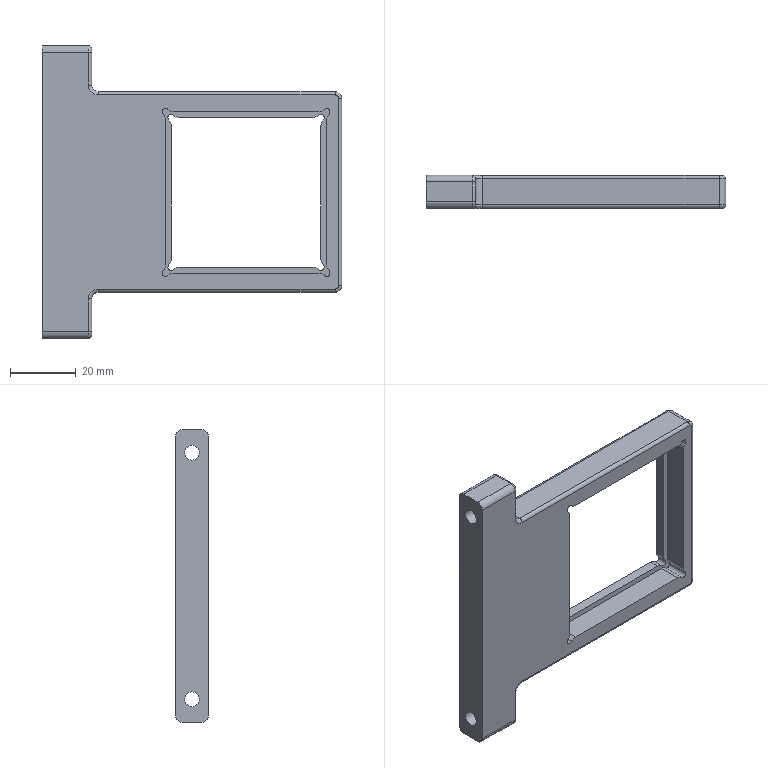NC program | NX | posted by the shop | part box 91 x 10 x 89 mm
Lines 2771 to 3778 of 16928:
N3 T04 M06
(D4  D=4. R=0. H=04 ce=0.05 di=0.05)
G00 G90 G54 X35.332 Y-21.985 M03 S6000
G43 H04 Z20.
M08
Z.31
G01 X35.333 Y-21.992 Z.225 F2000.
X35.336 Y-22.011 Z.147
X35.342 Y-22.04 Z.077
X35.35 Y-22.079 Z.014
X35.36 Y-22.124 Z-.041
X35.374 Y-22.175 Z-.09
X35.391 Y-22.229 Z-.133
X35.412 Y-22.285 Z-.17
X35.436 Y-22.341 Z-.201
X35.465 Y-22.395 Z-.226
X35.497 Y-22.446 Z-.247
X35.535 Y-22.491 Z-.263
X35.576 Y-22.529 Z-.275
X35.623 Y-22.559 Z-.283
X35.675 Y-22.578 Z-.288
X35.732 Y-22.585 Z-.29
X38.486 F2500.
G02 X38.904 Y-22.604 I0.0 J-4.55
X38.885 Y-22.185 I4.531 J.419
G01 Y-19.432
X38.869 Y-19.389
X38.823 Y-19.367 Z-.293
X38.751 Y-19.366 Z-.297
X38.656 Y-19.382 Z-.302
X38.541 Y-19.416 Z-.309
X38.411 Y-19.465 Z-.317
X38.267 Y-19.528 Z-.326
X38.115 Y-19.602 Z-.335
X37.956 Y-19.687 Z-.346
X37.795 Y-19.781 Z-.357
X37.635 Y-19.882 Z-.368
X37.298 Y-20.123 Z-.394
X36.982 Y-20.39 Z-.421
X36.691 Y-20.682 Z-.448
X36.423 Y-20.997 Z-.475
X36.182 Y-21.335 Z-.501
X36.081 Y-21.495 Z-.512
X35.987 Y-21.656 Z-.523
X35.903 Y-21.814 Z-.533
X35.828 Y-21.967 Z-.543
X35.765 Y-22.11 Z-.552
X35.717 Y-22.241 Z-.56
X35.683 Y-22.356 Z-.566
X35.666 Y-22.451 Z-.572
X35.667 Y-22.523 Z-.576
X35.689 Y-22.569 Z-.578
X35.732 Y-22.585 Z-.579
X38.486
G02 X38.904 Y-22.604 I0.0 J-4.55
X38.885 Y-22.185 I4.531 J.419
G01 Y-19.432
X38.869 Y-19.389 Z-.58
X38.823 Y-19.367 Z-.583
X38.751 Y-19.366 Z-.587
X38.656 Y-19.382 Z-.592
X38.541 Y-19.416 Z-.599
X38.411 Y-19.465 Z-.607
X38.267 Y-19.528 Z-.615
X38.115 Y-19.602 Z-.625
X37.956 Y-19.687 Z-.635
X37.795 Y-19.781 Z-.646
X37.635 Y-19.882 Z-.658
X37.298 Y-20.123 Z-.684
X36.982 Y-20.39 Z-.71
X36.691 Y-20.682 Z-.738
X36.423 Y-20.997 Z-.764
X36.182 Y-21.335 Z-.79
X36.081 Y-21.495 Z-.802
X35.987 Y-21.656 Z-.813
X35.903 Y-21.814 Z-.823
X35.828 Y-21.967 Z-.833
X35.765 Y-22.11 Z-.841
X35.717 Y-22.241 Z-.849
X35.683 Y-22.356 Z-.856
X35.666 Y-22.451 Z-.861
X35.667 Y-22.523 Z-.865
X35.689 Y-22.569 Z-.868
X35.732 Y-22.585 Z-.869
X38.486
G02 X38.904 Y-22.604 I0.0 J-4.55
X38.885 Y-22.185 I4.531 J.419
G01 Y-19.432
X38.869 Y-19.389 Z-.87
X38.823 Y-19.367 Z-.872
X38.751 Y-19.366 Z-.876
X38.656 Y-19.382 Z-.882
X38.541 Y-19.416 Z-.888
X38.411 Y-19.465 Z-.896
X38.267 Y-19.528 Z-.905
X38.115 Y-19.602 Z-.915
X37.956 Y-19.687 Z-.925
X37.795 Y-19.781 Z-.936
X37.635 Y-19.882 Z-.947
X37.298 Y-20.123 Z-.973
X36.982 Y-20.39 Z-1.
X36.691 Y-20.682 Z-1.027
X36.423 Y-20.997 Z-1.054
X36.182 Y-21.335 Z-1.08
X36.081 Y-21.495 Z-1.091
X35.987 Y-21.656 Z-1.102
X35.903 Y-21.814 Z-1.112
X35.828 Y-21.967 Z-1.122
X35.765 Y-22.11 Z-1.131
X35.717 Y-22.241 Z-1.139
X35.683 Y-22.356 Z-1.145
X35.666 Y-22.451 Z-1.151
X35.667 Y-22.523 Z-1.155
X35.689 Y-22.569 Z-1.157
X35.732 Y-22.585 Z-1.158
X38.486
G02 X38.904 Y-22.604 I0.0 J-4.55
X38.885 Y-22.185 I4.531 J.419
G01 Y-19.432
X38.869 Y-19.389 Z-1.159
X38.823 Y-19.367 Z-1.162
X38.751 Y-19.366 Z-1.166
X38.656 Y-19.382 Z-1.171
X38.541 Y-19.416 Z-1.178
X38.411 Y-19.465 Z-1.186
X38.267 Y-19.528 Z-1.195
X38.115 Y-19.602 Z-1.204
X37.956 Y-19.687 Z-1.215
X37.795 Y-19.781 Z-1.225
X37.635 Y-19.882 Z-1.237
X37.298 Y-20.123 Z-1.263
X36.982 Y-20.39 Z-1.29
X36.691 Y-20.682 Z-1.317
X36.423 Y-20.997 Z-1.344
X36.182 Y-21.335 Z-1.369
X36.081 Y-21.495 Z-1.381
X35.987 Y-21.656 Z-1.392
X35.903 Y-21.814 Z-1.402
X35.828 Y-21.967 Z-1.412
X35.765 Y-22.11 Z-1.421
X35.717 Y-22.241 Z-1.428
X35.683 Y-22.356 Z-1.435
X35.666 Y-22.451 Z-1.44
X35.667 Y-22.523 Z-1.445
X35.689 Y-22.569 Z-1.447
X35.732 Y-22.585 Z-1.448
X38.486
G02 X38.904 Y-22.604 I0.0 J-4.55
X38.885 Y-22.185 I4.531 J.419
G01 Y-19.432
X38.869 Y-19.389 Z-1.449
X38.823 Y-19.367 Z-1.451
X38.751 Y-19.366 Z-1.455
X38.656 Y-19.382 Z-1.461
X38.541 Y-19.416 Z-1.468
X38.411 Y-19.465 Z-1.475
X38.267 Y-19.528 Z-1.484
X38.115 Y-19.602 Z-1.494
X37.956 Y-19.687 Z-1.504
X37.795 Y-19.781 Z-1.515
X37.635 Y-19.882 Z-1.526
X37.298 Y-20.123 Z-1.552
X36.982 Y-20.39 Z-1.579
X36.691 Y-20.682 Z-1.606
X36.423 Y-20.997 Z-1.633
X36.182 Y-21.335 Z-1.659
X36.081 Y-21.495 Z-1.67
X35.987 Y-21.656 Z-1.681
X35.903 Y-21.814 Z-1.692
X35.828 Y-21.967 Z-1.701
X35.765 Y-22.11 Z-1.71
X35.717 Y-22.241 Z-1.718
X35.683 Y-22.356 Z-1.725
X35.666 Y-22.451 Z-1.73
X35.667 Y-22.523 Z-1.734
X35.689 Y-22.569 Z-1.737
X35.732 Y-22.585 Z-1.738
X38.486
G02 X38.904 Y-22.604 I0.0 J-4.55
X38.885 Y-22.185 I4.531 J.419
G01 Y-19.432
X38.869 Y-19.389
X38.823 Y-19.367 Z-1.741
X38.751 Y-19.366 Z-1.745
X38.656 Y-19.382 Z-1.75
X38.541 Y-19.416 Z-1.757
X38.411 Y-19.465 Z-1.765
X38.267 Y-19.528 Z-1.774
X38.115 Y-19.602 Z-1.783
X37.956 Y-19.687 Z-1.794
X37.795 Y-19.781 Z-1.805
X37.635 Y-19.882 Z-1.816
X37.298 Y-20.123 Z-1.842
X36.982 Y-20.39 Z-1.869
X36.691 Y-20.682 Z-1.896
X36.423 Y-20.997 Z-1.923
X36.182 Y-21.335 Z-1.949
X36.081 Y-21.495 Z-1.96
X35.987 Y-21.656 Z-1.971
X35.903 Y-21.814 Z-1.981
X35.828 Y-21.967 Z-1.991
X35.765 Y-22.11 Z-2.
X35.717 Y-22.241 Z-2.007
X35.683 Y-22.356 Z-2.014
X35.666 Y-22.451 Z-2.02
X35.667 Y-22.523 Z-2.024
X35.689 Y-22.569 Z-2.026
X35.732 Y-22.585 Z-2.027
X38.486
G02 X38.904 Y-22.604 I0.0 J-4.55
X38.885 Y-22.185 I4.531 J.419
G01 Y-19.432
X38.869 Y-19.389 Z-2.028
X38.823 Y-19.367 Z-2.03
X38.751 Y-19.366 Z-2.035
X38.656 Y-19.382 Z-2.04
X38.541 Y-19.416 Z-2.047
X38.411 Y-19.465 Z-2.054
X38.267 Y-19.528 Z-2.063
X38.115 Y-19.602 Z-2.073
X37.956 Y-19.687 Z-2.083
X37.795 Y-19.781 Z-2.094
X37.635 Y-19.882 Z-2.106
X37.298 Y-20.123 Z-2.131
X36.982 Y-20.39 Z-2.158
X36.691 Y-20.682 Z-2.185
X36.423 Y-20.997 Z-2.212
X36.182 Y-21.335 Z-2.238
X36.081 Y-21.495 Z-2.25
X35.987 Y-21.656 Z-2.26
X35.903 Y-21.814 Z-2.271
X35.828 Y-21.967 Z-2.28
X35.765 Y-22.11 Z-2.289
X35.717 Y-22.241 Z-2.297
X35.683 Y-22.356 Z-2.304
X35.666 Y-22.451 Z-2.309
X35.667 Y-22.523 Z-2.313
X35.689 Y-22.569 Z-2.316
X35.732 Y-22.585 Z-2.317
X38.486
G02 X38.904 Y-22.604 I0.0 J-4.55
X38.885 Y-22.185 I4.531 J.419
G01 Y-19.432
X38.869 Y-19.389 Z-2.318
X38.823 Y-19.367 Z-2.32
X38.751 Y-19.366 Z-2.324
X38.656 Y-19.382 Z-2.33
X38.541 Y-19.416 Z-2.336
X38.411 Y-19.465 Z-2.344
X38.267 Y-19.528 Z-2.353
X38.115 Y-19.602 Z-2.363
X37.956 Y-19.687 Z-2.373
X37.795 Y-19.781 Z-2.384
X37.635 Y-19.882 Z-2.395
X37.298 Y-20.123 Z-2.421
X36.982 Y-20.39 Z-2.448
X36.691 Y-20.682 Z-2.475
X36.423 Y-20.997 Z-2.502
X36.182 Y-21.335 Z-2.528
X36.081 Y-21.495 Z-2.539
X35.987 Y-21.656 Z-2.55
X35.903 Y-21.814 Z-2.56
X35.828 Y-21.967 Z-2.57
X35.765 Y-22.11 Z-2.579
X35.717 Y-22.241 Z-2.587
X35.683 Y-22.356 Z-2.593
X35.666 Y-22.451 Z-2.599
X35.667 Y-22.523 Z-2.603
X35.689 Y-22.569 Z-2.605
X35.732 Y-22.585 Z-2.606
X38.486
G02 X38.904 Y-22.604 I0.0 J-4.55
X38.885 Y-22.185 I4.531 J.419
G01 Y-19.432
X38.869 Y-19.389 Z-2.607
X38.823 Y-19.367 Z-2.61
X38.751 Y-19.366 Z-2.614
X38.656 Y-19.382 Z-2.619
X38.541 Y-19.416 Z-2.626
X38.411 Y-19.465 Z-2.634
X38.267 Y-19.528 Z-2.642
X38.115 Y-19.602 Z-2.652
X37.956 Y-19.687 Z-2.662
X37.795 Y-19.781 Z-2.673
X37.635 Y-19.882 Z-2.685
X37.298 Y-20.123 Z-2.711
X36.982 Y-20.39 Z-2.737
X36.691 Y-20.682 Z-2.765
X36.423 Y-20.997 Z-2.791
X36.182 Y-21.335 Z-2.817
X36.081 Y-21.495 Z-2.829
X35.987 Y-21.656 Z-2.84
X35.903 Y-21.814 Z-2.85
X35.828 Y-21.967 Z-2.86
X35.765 Y-22.11 Z-2.868
X35.717 Y-22.241 Z-2.876
X35.683 Y-22.356 Z-2.883
X35.666 Y-22.451 Z-2.888
X35.667 Y-22.523 Z-2.892
X35.689 Y-22.569 Z-2.895
X35.732 Y-22.585 Z-2.896
X38.486
G02 X38.904 Y-22.604 I0.0 J-4.55
X38.885 Y-22.185 I4.531 J.419
G01 Y-19.432
X38.869 Y-19.389 Z-2.897
X38.823 Y-19.367 Z-2.899
X38.751 Y-19.366 Z-2.903
X38.656 Y-19.382 Z-2.909
X38.541 Y-19.416 Z-2.915
X38.411 Y-19.465 Z-2.923
X38.267 Y-19.528 Z-2.932
X38.115 Y-19.602 Z-2.942
X37.956 Y-19.687 Z-2.952
X37.795 Y-19.781 Z-2.963
X37.635 Y-19.882 Z-2.974
X37.298 Y-20.123 Z-3.
X36.982 Y-20.39 Z-3.027
X36.691 Y-20.682 Z-3.054
X36.423 Y-20.997 Z-3.081
X36.182 Y-21.335 Z-3.107
X36.081 Y-21.495 Z-3.118
X35.987 Y-21.656 Z-3.129
X35.903 Y-21.814 Z-3.14
X35.828 Y-21.967 Z-3.149
X35.765 Y-22.11 Z-3.158
X35.717 Y-22.241 Z-3.166
X35.683 Y-22.356 Z-3.173
X35.666 Y-22.451 Z-3.178
X35.667 Y-22.523 Z-3.182
X35.689 Y-22.569 Z-3.185
X35.732 Y-22.585
X38.486
G02 X38.904 Y-22.604 I0.0 J-4.55
X38.885 Y-22.185 I4.531 J.419
G01 Y-19.432
X38.869 Y-19.389 Z-3.186
X38.823 Y-19.367 Z-3.189
X38.751 Y-19.366 Z-3.193
X38.656 Y-19.382 Z-3.198
X38.541 Y-19.416 Z-3.205
X38.411 Y-19.465 Z-3.213
X38.267 Y-19.528 Z-3.222
X38.115 Y-19.602 Z-3.231
X37.956 Y-19.687 Z-3.242
X37.795 Y-19.781 Z-3.253
X37.635 Y-19.882 Z-3.264
X37.298 Y-20.123 Z-3.29
X36.982 Y-20.39 Z-3.317
X36.691 Y-20.682 Z-3.344
X36.423 Y-20.997 Z-3.371
X36.182 Y-21.335 Z-3.397
X36.081 Y-21.495 Z-3.408
X35.987 Y-21.656 Z-3.419
X35.903 Y-21.814 Z-3.429
X35.828 Y-21.967 Z-3.439
X35.765 Y-22.11 Z-3.448
X35.717 Y-22.241 Z-3.455
X35.683 Y-22.356 Z-3.462
X35.666 Y-22.451 Z-3.468
X35.667 Y-22.523 Z-3.472
X35.689 Y-22.569 Z-3.474
X35.732 Y-22.585 Z-3.475
X38.486
G02 X38.904 Y-22.604 I0.0 J-4.55
X38.885 Y-22.185 I4.531 J.419
G01 Y-19.432
X38.869 Y-19.389 Z-3.476
X38.823 Y-19.367 Z-3.478
X38.751 Y-19.366 Z-3.482
X38.656 Y-19.382 Z-3.488
X38.541 Y-19.416 Z-3.495
X38.411 Y-19.465 Z-3.502
X38.267 Y-19.528 Z-3.511
X38.115 Y-19.602 Z-3.521
X37.956 Y-19.687 Z-3.531
X37.795 Y-19.781 Z-3.542
X37.635 Y-19.882 Z-3.553
X37.298 Y-20.123 Z-3.579
X36.982 Y-20.39 Z-3.606
X36.691 Y-20.682 Z-3.633
X36.423 Y-20.997 Z-3.66
X36.182 Y-21.335 Z-3.686
X36.081 Y-21.495 Z-3.698
X35.987 Y-21.656 Z-3.708
X35.903 Y-21.814 Z-3.719
X35.828 Y-21.967 Z-3.728
X35.765 Y-22.11 Z-3.737
X35.717 Y-22.241 Z-3.745
X35.683 Y-22.356 Z-3.752
X35.666 Y-22.451 Z-3.757
X35.667 Y-22.523 Z-3.761
X35.689 Y-22.569 Z-3.764
X35.732 Y-22.585 Z-3.765
X38.486
G02 X38.904 Y-22.604 I0.0 J-4.55
X38.885 Y-22.185 I4.531 J.419
G01 Y-19.432
X38.869 Y-19.389
X38.823 Y-19.367 Z-3.768
X38.751 Y-19.366 Z-3.772
X38.656 Y-19.382 Z-3.777
X38.541 Y-19.416 Z-3.784
X38.411 Y-19.465 Z-3.792
X38.267 Y-19.528 Z-3.801
X38.115 Y-19.602 Z-3.81
X37.956 Y-19.687 Z-3.821
X37.795 Y-19.781 Z-3.832
X37.635 Y-19.882 Z-3.843
X37.298 Y-20.123 Z-3.869
X36.982 Y-20.39 Z-3.896
X36.691 Y-20.682 Z-3.923
X36.423 Y-20.997 Z-3.95
X36.182 Y-21.335 Z-3.976
X36.081 Y-21.495 Z-3.987
X35.987 Y-21.656 Z-3.998
X35.903 Y-21.814 Z-4.008
X35.828 Y-21.967 Z-4.018
X35.765 Y-22.11 Z-4.027
X35.717 Y-22.241 Z-4.035
X35.683 Y-22.356 Z-4.041
X35.666 Y-22.451 Z-4.047
X35.667 Y-22.523 Z-4.051
X35.689 Y-22.569 Z-4.053
X35.732 Y-22.585 Z-4.054
X38.486
G02 X38.904 Y-22.604 I0.0 J-4.55
X38.885 Y-22.185 I4.531 J.419
G01 Y-19.432
X38.869 Y-19.389 Z-4.055
X38.823 Y-19.367 Z-4.058
X38.751 Y-19.366 Z-4.062
X38.656 Y-19.382 Z-4.067
X38.541 Y-19.416 Z-4.074
X38.411 Y-19.465 Z-4.082
X38.267 Y-19.528 Z-4.09
X38.115 Y-19.602 Z-4.1
X37.956 Y-19.687 Z-4.11
X37.795 Y-19.781 Z-4.121
X37.635 Y-19.882 Z-4.133
X37.298 Y-20.123 Z-4.159
X36.982 Y-20.39 Z-4.185
X36.691 Y-20.682 Z-4.213
X36.423 Y-20.997 Z-4.239
X36.182 Y-21.335 Z-4.265
X36.081 Y-21.495 Z-4.277
X35.987 Y-21.656 Z-4.288
X35.903 Y-21.814 Z-4.298
X35.828 Y-21.967 Z-4.308
X35.765 Y-22.11 Z-4.316
X35.717 Y-22.241 Z-4.324
X35.683 Y-22.356 Z-4.331
X35.666 Y-22.451 Z-4.336
X35.667 Y-22.523 Z-4.34
X35.689 Y-22.569 Z-4.343
X35.732 Y-22.585 Z-4.344
X38.486
G02 X38.904 Y-22.604 I0.0 J-4.55
X38.885 Y-22.185 I4.531 J.419
G01 Y-19.432
X38.869 Y-19.389 Z-4.345
X38.823 Y-19.367 Z-4.347
X38.751 Y-19.366 Z-4.351
X38.656 Y-19.382 Z-4.357
X38.541 Y-19.416 Z-4.363
X38.411 Y-19.465 Z-4.371
X38.267 Y-19.528 Z-4.38
X38.115 Y-19.602 Z-4.39
X37.956 Y-19.687 Z-4.4
X37.795 Y-19.781 Z-4.411
X37.635 Y-19.882 Z-4.422
X37.298 Y-20.123 Z-4.448
X36.982 Y-20.39 Z-4.475
X36.691 Y-20.682 Z-4.502
X36.423 Y-20.997 Z-4.529
X36.182 Y-21.335 Z-4.555
X36.081 Y-21.495 Z-4.566
X35.987 Y-21.656 Z-4.577
X35.903 Y-21.814 Z-4.587
X35.828 Y-21.967 Z-4.597
X35.765 Y-22.11 Z-4.606
X35.717 Y-22.241 Z-4.614
X35.683 Y-22.356 Z-4.62
X35.666 Y-22.451 Z-4.626
X35.667 Y-22.523 Z-4.63
X35.689 Y-22.569 Z-4.632
X35.732 Y-22.585 Z-4.633
X38.486
G02 X38.904 Y-22.604 I0.0 J-4.55
X38.885 Y-22.185 I4.531 J.419
G01 Y-19.432
X38.869 Y-19.389 Z-4.634
X38.823 Y-19.367 Z-4.637
X38.751 Y-19.366 Z-4.641
X38.656 Y-19.382 Z-4.646
X38.541 Y-19.416 Z-4.653
X38.411 Y-19.465 Z-4.661
X38.267 Y-19.528 Z-4.67
X38.115 Y-19.602 Z-4.679
X37.956 Y-19.687 Z-4.69
X37.795 Y-19.781 Z-4.7
X37.635 Y-19.882 Z-4.712
X37.298 Y-20.123 Z-4.738
X36.982 Y-20.39 Z-4.765
X36.691 Y-20.682 Z-4.792
X36.423 Y-20.997 Z-4.819
X36.182 Y-21.335 Z-4.844
X36.081 Y-21.495 Z-4.856
X35.987 Y-21.656 Z-4.867
X35.903 Y-21.814 Z-4.877
X35.828 Y-21.967 Z-4.887
X35.765 Y-22.11 Z-4.896
X35.717 Y-22.241 Z-4.903
X35.683 Y-22.356 Z-4.91
X35.666 Y-22.451 Z-4.915
X35.667 Y-22.523 Z-4.92
X35.689 Y-22.569 Z-4.922
X35.732 Y-22.585 Z-4.923
X38.486
G02 X38.904 Y-22.604 I0.0 J-4.55
X38.885 Y-22.185 I4.531 J.419
G01 Y-19.432
X38.869 Y-19.389 Z-4.924
X38.823 Y-19.367 Z-4.926
X38.751 Y-19.366 Z-4.93
X38.656 Y-19.382 Z-4.936
X38.541 Y-19.416 Z-4.943
X38.411 Y-19.465 Z-4.95
X38.267 Y-19.528 Z-4.959
X38.115 Y-19.602 Z-4.969
X37.956 Y-19.687 Z-4.979
X37.795 Y-19.781 Z-4.99
X37.635 Y-19.882 Z-5.001
X37.298 Y-20.123 Z-5.027
X36.982 Y-20.39 Z-5.054
X36.691 Y-20.682 Z-5.081
X36.423 Y-20.997 Z-5.108
X36.182 Y-21.335 Z-5.134
X36.081 Y-21.495 Z-5.145
X35.987 Y-21.656 Z-5.156
X35.903 Y-21.814 Z-5.167
X35.828 Y-21.967 Z-5.176
X35.765 Y-22.11 Z-5.185
X35.717 Y-22.241 Z-5.193
X35.683 Y-22.356 Z-5.2
X35.666 Y-22.451 Z-5.205
X35.667 Y-22.523 Z-5.209
X35.689 Y-22.569 Z-5.212
X35.732 Y-22.585 Z-5.213
X38.486
G02 X38.904 Y-22.604 I0.0 J-4.55
X38.885 Y-22.185 I4.531 J.419
G01 Y-19.432
X38.869 Y-19.389
X38.823 Y-19.367 Z-5.216
X38.751 Y-19.366 Z-5.22
X38.656 Y-19.382 Z-5.225
X38.541 Y-19.416 Z-5.232
X38.411 Y-19.465 Z-5.24
X38.267 Y-19.528 Z-5.249
X38.115 Y-19.602 Z-5.258
X37.956 Y-19.687 Z-5.269
X37.795 Y-19.781 Z-5.28
X37.635 Y-19.882 Z-5.291
X37.298 Y-20.123 Z-5.317
X36.982 Y-20.39 Z-5.344
X36.691 Y-20.682 Z-5.371
X36.423 Y-20.997 Z-5.398
X36.182 Y-21.335 Z-5.424
X36.081 Y-21.495 Z-5.435
X35.987 Y-21.656 Z-5.446
X35.903 Y-21.814 Z-5.456
X35.828 Y-21.967 Z-5.466
X35.765 Y-22.11 Z-5.475
X35.717 Y-22.241 Z-5.482
X35.683 Y-22.356 Z-5.489
X35.666 Y-22.451 Z-5.495
X35.667 Y-22.523 Z-5.499
X35.689 Y-22.569 Z-5.501
X35.732 Y-22.585 Z-5.502
X38.486
G02 X38.904 Y-22.604 I0.0 J-4.55
X38.885 Y-22.185 I4.531 J.419
G01 Y-19.432
X38.869 Y-19.389 Z-5.503
X38.823 Y-19.367 Z-5.505
X38.751 Y-19.366 Z-5.51
X38.656 Y-19.382 Z-5.515
X38.541 Y-19.416 Z-5.522
X38.411 Y-19.465 Z-5.529
X38.267 Y-19.528 Z-5.538
X38.115 Y-19.602 Z-5.548
X37.956 Y-19.687 Z-5.558
X37.795 Y-19.781 Z-5.569
X37.635 Y-19.882 Z-5.581
X37.298 Y-20.123 Z-5.606
X36.982 Y-20.39 Z-5.633
X36.691 Y-20.682 Z-5.66
X36.423 Y-20.997 Z-5.687
X36.182 Y-21.335 Z-5.713
X36.081 Y-21.495 Z-5.725
X35.987 Y-21.656 Z-5.735
X35.903 Y-21.814 Z-5.746
X35.828 Y-21.967 Z-5.755
X35.765 Y-22.11 Z-5.764
X35.717 Y-22.241 Z-5.772
X35.683 Y-22.356 Z-5.779
X35.666 Y-22.451 Z-5.784
X35.667 Y-22.523 Z-5.788
X35.689 Y-22.569 Z-5.791
X35.732 Y-22.585 Z-5.792
X38.486
G02 X38.904 Y-22.604 I0.0 J-4.55
X38.885 Y-22.185 I4.531 J.419
G01 Y-19.432
X38.869 Y-19.389 Z-5.793
X38.823 Y-19.367 Z-5.795
X38.751 Y-19.366 Z-5.799
X38.656 Y-19.382 Z-5.805
X38.541 Y-19.416 Z-5.811
X38.411 Y-19.465 Z-5.819
X38.267 Y-19.528 Z-5.828
X38.115 Y-19.602 Z-5.838
X37.956 Y-19.687 Z-5.848
X37.795 Y-19.781 Z-5.859
X37.635 Y-19.882 Z-5.87
X37.298 Y-20.123 Z-5.896
X36.982 Y-20.39 Z-5.923
X36.691 Y-20.682 Z-5.95
X36.423 Y-20.997 Z-5.977
X36.182 Y-21.335 Z-6.003
X36.081 Y-21.495 Z-6.014
X35.987 Y-21.656 Z-6.025
X35.903 Y-21.814 Z-6.035
X35.828 Y-21.967 Z-6.045
X35.765 Y-22.11 Z-6.054
X35.717 Y-22.241 Z-6.062
X35.683 Y-22.356 Z-6.068
X35.666 Y-22.451 Z-6.074
X35.667 Y-22.523 Z-6.078
X35.689 Y-22.569 Z-6.08
X35.732 Y-22.585 Z-6.081
X38.486
G02 X38.904 Y-22.604 I0.0 J-4.55
X38.885 Y-22.185 I4.531 J.419
G01 Y-19.432
X38.869 Y-19.389 Z-6.082
X38.823 Y-19.367 Z-6.085
X38.751 Y-19.366 Z-6.089
X38.656 Y-19.382 Z-6.094
X38.541 Y-19.416 Z-6.101
X38.411 Y-19.465 Z-6.109
X38.267 Y-19.528 Z-6.117
X38.115 Y-19.602 Z-6.127
X37.956 Y-19.687 Z-6.137
X37.795 Y-19.781 Z-6.148
X37.635 Y-19.882 Z-6.16
X37.298 Y-20.123 Z-6.186
X36.982 Y-20.39 Z-6.212
X36.691 Y-20.682 Z-6.24
X36.423 Y-20.997 Z-6.266
X36.182 Y-21.335 Z-6.292
X36.081 Y-21.495 Z-6.304
X35.987 Y-21.656 Z-6.315
X35.903 Y-21.814 Z-6.325
X35.828 Y-21.967 Z-6.335
X35.765 Y-22.11 Z-6.343
X35.717 Y-22.241 Z-6.351
X35.683 Y-22.356 Z-6.358
X35.666 Y-22.451 Z-6.363
X35.667 Y-22.523 Z-6.367
X35.689 Y-22.569 Z-6.37
X35.732 Y-22.585 Z-6.371
X38.486
G02 X38.904 Y-22.604 I0.0 J-4.55
X38.885 Y-22.185 I4.531 J.419
G01 Y-19.432
X38.869 Y-19.389 Z-6.372
X38.823 Y-19.367 Z-6.374
X38.751 Y-19.366 Z-6.378
X38.656 Y-19.382 Z-6.384
X38.541 Y-19.416 Z-6.39
X38.411 Y-19.465 Z-6.398
X38.267 Y-19.528 Z-6.407
X38.115 Y-19.602 Z-6.417
X37.956 Y-19.687 Z-6.427
X37.795 Y-19.781 Z-6.438
X37.635 Y-19.882 Z-6.449
X37.298 Y-20.123 Z-6.475
X36.982 Y-20.39 Z-6.502
X36.691 Y-20.682 Z-6.529
X36.423 Y-20.997 Z-6.556
X36.182 Y-21.335 Z-6.582
X36.081 Y-21.495 Z-6.593
X35.987 Y-21.656 Z-6.604
X35.903 Y-21.814 Z-6.615
X35.828 Y-21.967 Z-6.624
X35.765 Y-22.11 Z-6.633
X35.717 Y-22.241 Z-6.641
X35.683 Y-22.356 Z-6.648
X35.666 Y-22.451 Z-6.653
X35.667 Y-22.523 Z-6.657
X35.689 Y-22.569 Z-6.66
X35.732 Y-22.585
X38.486
G02 X38.904 Y-22.604 I0.0 J-4.55
X38.885 Y-22.185 I4.531 J.419
G01 Y-19.432
X38.869 Y-19.389 Z-6.661
X38.823 Y-19.367 Z-6.664
X38.751 Y-19.366 Z-6.668
X38.656 Y-19.382 Z-6.673
X38.541 Y-19.416 Z-6.68
X38.411 Y-19.465 Z-6.688
X38.267 Y-19.528 Z-6.697
X38.115 Y-19.602 Z-6.706
X37.956 Y-19.687 Z-6.717
X37.795 Y-19.781 Z-6.728
X37.635 Y-19.882 Z-6.739
X37.298 Y-20.123 Z-6.765
X36.982 Y-20.39 Z-6.792
X36.691 Y-20.682 Z-6.819
X36.423 Y-20.997 Z-6.846
X36.182 Y-21.335 Z-6.872
X36.081 Y-21.495 Z-6.883
X35.987 Y-21.656 Z-6.894
X35.903 Y-21.814 Z-6.904
X35.828 Y-21.967 Z-6.914
X35.765 Y-22.11 Z-6.923
X35.717 Y-22.241 Z-6.93
X35.683 Y-22.356 Z-6.937
X35.666 Y-22.451 Z-6.943
X35.667 Y-22.523 Z-6.947
X35.689 Y-22.569 Z-6.949
X35.732 Y-22.585 Z-6.95
X38.486
G02 X38.904 Y-22.604 I0.0 J-4.55
X38.885 Y-22.185 I4.531 J.419
G01 Y-19.432
X38.878 Y-19.375 Z-6.949
X38.859 Y-19.323 Z-6.944
X38.83 Y-19.276 Z-6.936
X38.791 Y-19.234 Z-6.924
X38.746 Y-19.197 Z-6.908
X38.695 Y-19.165 Z-6.887
X38.641 Y-19.136 Z-6.861
X38.585 Y-19.112 Z-6.83
X38.529 Y-19.091 Z-6.793
X38.475 Y-19.074 Z-6.751
X38.424 Y-19.06 Z-6.702
X38.379 Y-19.049 Z-6.646
X38.34 Y-19.041 Z-6.584
X38.311 Y-19.036 Z-6.514
X38.292 Y-19.033 Z-6.436
X38.285 Y-19.032 Z-6.35
G00 Z3.
Y18.762
Z.31
G01 X38.292 Y18.763 Z.225 F2000.
X38.311 Y18.766 Z.147
X38.34 Y18.772 Z.077
X38.379 Y18.78 Z.014
X38.424 Y18.791 Z-.041
X38.475 Y18.804 Z-.09
X38.529 Y18.822 Z-.133
X38.585 Y18.842 Z-.17
X38.641 Y18.867 Z-.201
X38.695 Y18.895 Z-.226
X38.746 Y18.928 Z-.247
X38.791 Y18.965 Z-.263
X38.83 Y19.006 Z-.275
X38.859 Y19.053 Z-.283
X38.878 Y19.105 Z-.288
X38.885 Y19.162 Z-.29
Y21.916 F2500.
G02 X38.904 Y22.335 I4.55 J0.0
X38.486 Y22.315 I-.419 J4.531
G01 X35.732
X35.689 Y22.299
X35.667 Y22.253 Z-.293
X35.666 Y22.181 Z-.297
X35.683 Y22.086 Z-.302
X35.717 Y21.972 Z-.309
X35.765 Y21.841 Z-.317
X35.828 Y21.698 Z-.326
X35.903 Y21.545 Z-.335
X35.987 Y21.386 Z-.346
X36.081 Y21.225 Z-.357
X36.182 Y21.065 Z-.368
X36.423 Y20.728 Z-.394
X36.691 Y20.413 Z-.421
X36.982 Y20.121 Z-.448
X37.298 Y19.854 Z-.475
X37.635 Y19.612 Z-.501
X37.795 Y19.511 Z-.512
X37.956 Y19.418 Z-.523
X38.115 Y19.333 Z-.533
X38.267 Y19.258 Z-.543
X38.411 Y19.196 Z-.552
X38.541 Y19.147 Z-.56
X38.656 Y19.113 Z-.566
X38.751 Y19.096 Z-.572
X38.823 Y19.097 Z-.576
X38.869 Y19.119 Z-.578
X38.885 Y19.162 Z-.579
Y21.916
G02 X38.904 Y22.335 I4.55 J0.0
X38.486 Y22.315 I-.419 J4.531
G01 X35.732
X35.689 Y22.299 Z-.58
X35.667 Y22.253 Z-.583
X35.666 Y22.181 Z-.587
X35.683 Y22.086 Z-.592
X35.717 Y21.972 Z-.599
X35.765 Y21.841 Z-.607
X35.828 Y21.698 Z-.615
X35.903 Y21.545 Z-.625
X35.987 Y21.386 Z-.635
X36.081 Y21.225 Z-.646
X36.182 Y21.065 Z-.658
X36.423 Y20.728 Z-.684
X36.691 Y20.413 Z-.71
X36.982 Y20.121 Z-.738
X37.298 Y19.854 Z-.764
X37.635 Y19.612 Z-.79
X37.795 Y19.511 Z-.802
X37.956 Y19.418 Z-.813
X38.115 Y19.333 Z-.823
X38.267 Y19.258 Z-.833
X38.411 Y19.196 Z-.841
X38.541 Y19.147 Z-.849
X38.656 Y19.113 Z-.856
X38.751 Y19.096 Z-.861
X38.823 Y19.097 Z-.865
X38.869 Y19.119 Z-.868
X38.885 Y19.162 Z-.869
Y21.916
G02 X38.904 Y22.335 I4.55 J0.0
X38.486 Y22.315 I-.419 J4.531
G01 X35.732
X35.689 Y22.299 Z-.87
X35.667 Y22.253 Z-.872
X35.666 Y22.181 Z-.876
X35.683 Y22.086 Z-.882
X35.717 Y21.972 Z-.888
X35.765 Y21.841 Z-.896
X35.828 Y21.698 Z-.905
X35.903 Y21.545 Z-.915
X35.987 Y21.386 Z-.925
X36.081 Y21.225 Z-.936
X36.182 Y21.065 Z-.947
X36.423 Y20.728 Z-.973
X36.691 Y20.413 Z-1.
X36.982 Y20.121 Z-1.027
X37.298 Y19.854 Z-1.054
X37.635 Y19.612 Z-1.08
X37.795 Y19.511 Z-1.091
X37.956 Y19.418 Z-1.102
X38.115 Y19.333 Z-1.112
X38.267 Y19.258 Z-1.122
X38.411 Y19.196 Z-1.131
X38.541 Y19.147 Z-1.139
X38.656 Y19.113 Z-1.145
X38.751 Y19.096 Z-1.151
X38.823 Y19.097 Z-1.155
X38.869 Y19.119 Z-1.157
X38.885 Y19.162 Z-1.158
Y21.916
G02 X38.904 Y22.335 I4.55 J0.0
X38.486 Y22.315 I-.419 J4.531
G01 X35.732
X35.689 Y22.299 Z-1.159
X35.667 Y22.253 Z-1.162
X35.666 Y22.181 Z-1.166
X35.683 Y22.086 Z-1.171
X35.717 Y21.972 Z-1.178
X35.765 Y21.841 Z-1.186
X35.828 Y21.698 Z-1.195
X35.903 Y21.545 Z-1.204
X35.987 Y21.386 Z-1.215
X36.081 Y21.225 Z-1.225
X36.182 Y21.065 Z-1.237
X36.423 Y20.728 Z-1.263
X36.691 Y20.413 Z-1.29
X36.982 Y20.121 Z-1.317
X37.298 Y19.854 Z-1.344
X37.635 Y19.612 Z-1.369
X37.795 Y19.511 Z-1.381
X37.956 Y19.418 Z-1.392
X38.115 Y19.333 Z-1.402
X38.267 Y19.258 Z-1.412
X38.411 Y19.196 Z-1.421
X38.541 Y19.147 Z-1.428
X38.656 Y19.113 Z-1.435
X38.751 Y19.096 Z-1.44
X38.823 Y19.097 Z-1.445
X38.869 Y19.119 Z-1.447
X38.885 Y19.162 Z-1.448
Y21.916
G02 X38.904 Y22.335 I4.55 J0.0
X38.486 Y22.315 I-.419 J4.531
G01 X35.732
X35.689 Y22.299 Z-1.449
X35.667 Y22.253 Z-1.451
X35.666 Y22.181 Z-1.455
X35.683 Y22.086 Z-1.461
X35.717 Y21.972 Z-1.468
X35.765 Y21.841 Z-1.475
X35.828 Y21.698 Z-1.484
X35.903 Y21.545 Z-1.494
X35.987 Y21.386 Z-1.504
X36.081 Y21.225 Z-1.515
X36.182 Y21.065 Z-1.526
X36.423 Y20.728 Z-1.552
X36.691 Y20.413 Z-1.579
X36.982 Y20.121 Z-1.606
X37.298 Y19.854 Z-1.633
X37.635 Y19.612 Z-1.659
X37.795 Y19.511 Z-1.67
X37.956 Y19.418 Z-1.681
X38.115 Y19.333 Z-1.692
X38.267 Y19.258 Z-1.701
X38.411 Y19.196 Z-1.71
X38.541 Y19.147 Z-1.718
X38.656 Y19.113 Z-1.725
X38.751 Y19.096 Z-1.73
X38.823 Y19.097 Z-1.734
X38.869 Y19.119 Z-1.737
X38.885 Y19.162 Z-1.738
Y21.916
G02 X38.904 Y22.335 I4.55 J0.0
X38.486 Y22.315 I-.419 J4.531
G01 X35.732
X35.689 Y22.299
X35.667 Y22.253 Z-1.741
X35.666 Y22.181 Z-1.745
X35.683 Y22.086 Z-1.75
X35.717 Y21.972 Z-1.757
X35.765 Y21.841 Z-1.765
X35.828 Y21.698 Z-1.774
X35.903 Y21.545 Z-1.783
X35.987 Y21.386 Z-1.794
X36.081 Y21.225 Z-1.805
X36.182 Y21.065 Z-1.816
X36.423 Y20.728 Z-1.842
X36.691 Y20.413 Z-1.869
X36.982 Y20.121 Z-1.896
X37.298 Y19.854 Z-1.923
X37.635 Y19.612 Z-1.949
X37.795 Y19.511 Z-1.96
X37.956 Y19.418 Z-1.971
X38.115 Y19.333 Z-1.981
X38.267 Y19.258 Z-1.991
X38.411 Y19.196 Z-2.
X38.541 Y19.147 Z-2.007
X38.656 Y19.113 Z-2.014
X38.751 Y19.096 Z-2.02
X38.823 Y19.097 Z-2.024
X38.869 Y19.119 Z-2.026
X38.885 Y19.162 Z-2.027
Y21.916
G02 X38.904 Y22.335 I4.55 J0.0
X38.486 Y22.315 I-.419 J4.531
G01 X35.732
X35.689 Y22.299 Z-2.028
X35.667 Y22.253 Z-2.03
X35.666 Y22.181 Z-2.035
X35.683 Y22.086 Z-2.04
X35.717 Y21.972 Z-2.047
X35.765 Y21.841 Z-2.054
X35.828 Y21.698 Z-2.063
X35.903 Y21.545 Z-2.073
X35.987 Y21.386 Z-2.083
X36.081 Y21.225 Z-2.094
X36.182 Y21.065 Z-2.106
X36.423 Y20.728 Z-2.131
X36.691 Y20.413 Z-2.158
X36.982 Y20.121 Z-2.185
X37.298 Y19.854 Z-2.212
X37.635 Y19.612 Z-2.238
X37.795 Y19.511 Z-2.25
X37.956 Y19.418 Z-2.26
X38.115 Y19.333 Z-2.271
X38.267 Y19.258 Z-2.28
X38.411 Y19.196 Z-2.289
X38.541 Y19.147 Z-2.297
X38.656 Y19.113 Z-2.304
X38.751 Y19.096 Z-2.309
X38.823 Y19.097 Z-2.313
X38.869 Y19.119 Z-2.316
X38.885 Y19.162 Z-2.317
Y21.916
G02 X38.904 Y22.335 I4.55 J0.0
X38.486 Y22.315 I-.419 J4.531
G01 X35.732
X35.689 Y22.299 Z-2.318
X35.667 Y22.253 Z-2.32
X35.666 Y22.181 Z-2.324
X35.683 Y22.086 Z-2.33
X35.717 Y21.972 Z-2.336
X35.765 Y21.841 Z-2.344
X35.828 Y21.698 Z-2.353
X35.903 Y21.545 Z-2.363
X35.987 Y21.386 Z-2.373
X36.081 Y21.225 Z-2.384
X36.182 Y21.065 Z-2.395
X36.423 Y20.728 Z-2.421
X36.691 Y20.413 Z-2.448